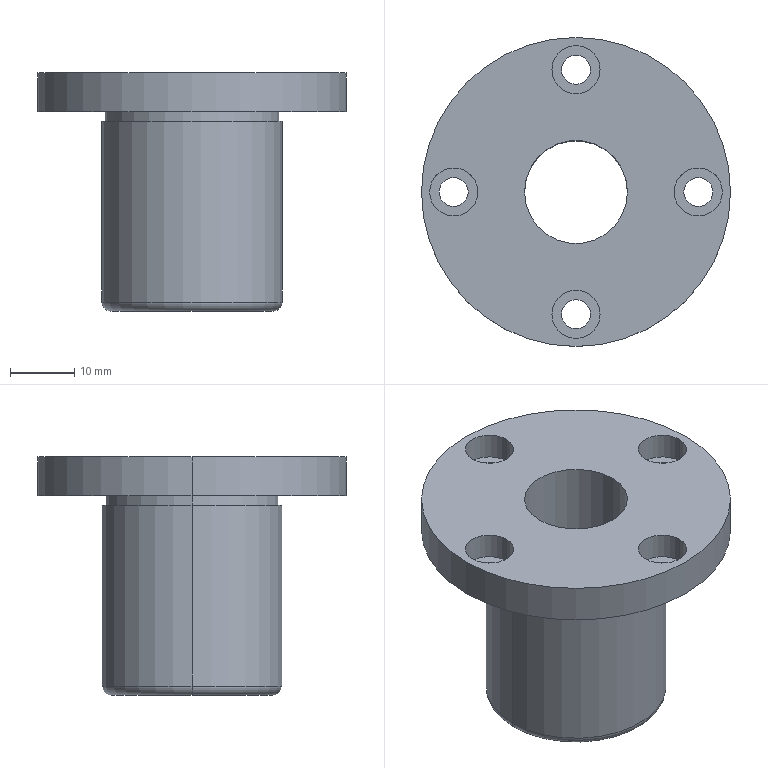Part | SolidWorks | features BaseBody 1 | 1 solid | 34 faces | box 48 x 48 x 37 mm | volume 21560 mm3 | cylinder 24 | plane 8 | torus 2 | commonest cylinder face diameters 4.5 x8 7.5 x8 16 x2 27 x2 28 x2 48 x2
STEP:
#1=CARTESIAN_POINT('',(-611.131,726.211,541.732));
#2=VERTEX_POINT('',#1);
#3=CARTESIAN_POINT('',(-595.131,726.211,541.732));
#4=VERTEX_POINT('',#3);
#5=CARTESIAN_POINT('',(-603.131,726.211,541.732));
#6=DIRECTION('',(0.,0.,1.));
#7=DIRECTION('',(-1.,0.,0.));
#8=AXIS2_PLACEMENT_3D('',#5,#6,#7);
#9=CIRCLE('',#8,8.);
#10=EDGE_CURVE('',#2,#4,#9,.T.);
#11=ORIENTED_EDGE('',*,*,#10,.T.);
#12=CARTESIAN_POINT('',(-595.131,726.211,504.732));
#13=VERTEX_POINT('',#12);
#14=CARTESIAN_POINT('',(-595.131,726.211,504.732));
#15=DIRECTION('',(0.,0.,1.));
#16=VECTOR('',#15,1000.);
#17=LINE('',#14,#16);
#18=EDGE_CURVE('',#13,#4,#17,.T.);
#19=ORIENTED_EDGE('',*,*,#18,.F.);
#20=CARTESIAN_POINT('',(-611.131,726.211,504.732));
#21=VERTEX_POINT('',#20);
#22=CARTESIAN_POINT('',(-603.131,726.211,504.732));
#23=DIRECTION('',(0.,0.,-1.));
#24=DIRECTION('',(1.,0.,0.));
#25=AXIS2_PLACEMENT_3D('',#22,#23,#24);
#26=CIRCLE('',#25,8.);
#27=EDGE_CURVE('',#13,#21,#26,.T.);
#28=ORIENTED_EDGE('',*,*,#27,.T.);
#29=CARTESIAN_POINT('',(-611.131,726.211,541.732));
#30=DIRECTION('',(0.,0.,-1.));
#31=VECTOR('',#30,1000.);
#32=LINE('',#29,#31);
#33=EDGE_CURVE('',#2,#21,#32,.T.);
#34=ORIENTED_EDGE('',*,*,#33,.F.);
#35=EDGE_LOOP('',(#11,#19,#28,#34));
#36=FACE_OUTER_BOUND('',#35,.T.);
#37=CARTESIAN_POINT('',(-603.131,726.211,504.732));
#38=DIRECTION('',(0.,0.,1.));
#39=DIRECTION('',(-1.,0.,0.));
#40=AXIS2_PLACEMENT_3D('',#37,#38,#39);
#41=CYLINDRICAL_SURFACE('',#40,8.);
#42=ADVANCED_FACE('',(#36),#41,.F.);
#43=ORIENTED_EDGE('',*,*,#18,.T.);
#44=CARTESIAN_POINT('',(-603.131,726.211,541.732));
#45=DIRECTION('',(0.,0.,1.));
#46=DIRECTION('',(1.,0.,0.));
#47=AXIS2_PLACEMENT_3D('',#44,#45,#46);
#48=CIRCLE('',#47,8.);
#49=EDGE_CURVE('',#4,#2,#48,.T.);
#50=ORIENTED_EDGE('',*,*,#49,.T.);
#51=ORIENTED_EDGE('',*,*,#33,.T.);
#52=CARTESIAN_POINT('',(-603.131,726.211,504.732));
#53=DIRECTION('',(0.,0.,-1.));
#54=DIRECTION('',(-1.,0.,0.));
#55=AXIS2_PLACEMENT_3D('',#52,#53,#54);
#56=CIRCLE('',#55,8.);
#57=EDGE_CURVE('',#21,#13,#56,.T.);
#58=ORIENTED_EDGE('',*,*,#57,.T.);
#59=EDGE_LOOP('',(#43,#50,#51,#58));
#60=FACE_OUTER_BOUND('',#59,.T.);
#61=CARTESIAN_POINT('',(-603.131,726.211,504.732));
#62=DIRECTION('',(0.,0.,1.));
#63=DIRECTION('',(-1.,0.,0.));
#64=AXIS2_PLACEMENT_3D('',#61,#62,#63);
#65=CYLINDRICAL_SURFACE('',#64,8.);
#66=ADVANCED_FACE('',(#60),#65,.F.);
#67=CARTESIAN_POINT('',(-590.531,726.211,504.732));
#68=VERTEX_POINT('',#67);
#69=CARTESIAN_POINT('',(-615.731,726.211,504.732));
#70=VERTEX_POINT('',#69);
#71=CARTESIAN_POINT('',(-603.131,726.211,504.732));
#72=DIRECTION('',(0.,0.,1.));
#73=DIRECTION('',(1.,0.,0.));
#74=AXIS2_PLACEMENT_3D('',#71,#72,#73);
#75=CIRCLE('',#74,12.6);
#76=EDGE_CURVE('',#68,#70,#75,.T.);
#77=ORIENTED_EDGE('',*,*,#76,.F.);
#78=CARTESIAN_POINT('',(-603.131,726.211,504.732));
#79=DIRECTION('',(0.,0.,1.));
#80=DIRECTION('',(-1.,0.,0.));
#81=AXIS2_PLACEMENT_3D('',#78,#79,#80);
#82=CIRCLE('',#81,12.6);
#83=EDGE_CURVE('',#70,#68,#82,.T.);
#84=ORIENTED_EDGE('',*,*,#83,.F.);
#85=EDGE_LOOP('',(#77,#84));
#86=FACE_OUTER_BOUND('',#85,.T.);
#87=ORIENTED_EDGE('',*,*,#57,.F.);
#88=ORIENTED_EDGE('',*,*,#27,.F.);
#89=EDGE_LOOP('',(#87,#88));
#90=FACE_BOUND('',#89,.T.);
#91=CARTESIAN_POINT('',(-603.131,734.211,504.732));
#92=DIRECTION('',(0.,0.,1.));
#93=DIRECTION('',(-1.,0.,0.));
#94=AXIS2_PLACEMENT_3D('',#91,#92,#93);
#95=PLANE('',#94);
#96=ADVANCED_FACE('',(#86,#90),#95,.F.);
#97=CARTESIAN_POINT('',(-589.131,726.211,506.132));
#98=VERTEX_POINT('',#97);
#99=CARTESIAN_POINT('',(-590.531,726.211,506.132));
#100=DIRECTION('',(0.,-1.,0.));
#101=DIRECTION('',(0.,0.,-1.));
#102=AXIS2_PLACEMENT_3D('',#99,#100,#101);
#103=CIRCLE('',#102,1.4);
#104=EDGE_CURVE('',#68,#98,#103,.T.);
#105=ORIENTED_EDGE('',*,*,#104,.T.);
#106=CARTESIAN_POINT('',(-617.131,726.211,506.132));
#107=VERTEX_POINT('',#106);
#108=CARTESIAN_POINT('',(-603.131,726.211,506.132));
#109=DIRECTION('',(0.,0.,1.));
#110=DIRECTION('',(-1.,0.,0.));
#111=AXIS2_PLACEMENT_3D('',#108,#109,#110);
#112=CIRCLE('',#111,14.);
#113=EDGE_CURVE('',#107,#98,#112,.T.);
#114=ORIENTED_EDGE('',*,*,#113,.F.);
#115=CARTESIAN_POINT('',(-615.731,726.211,506.132));
#116=DIRECTION('',(0.,-1.,0.));
#117=DIRECTION('',(-1.,0.,0.));
#118=AXIS2_PLACEMENT_3D('',#115,#116,#117);
#119=CIRCLE('',#118,1.4);
#120=EDGE_CURVE('',#107,#70,#119,.T.);
#121=ORIENTED_EDGE('',*,*,#120,.T.);
#122=ORIENTED_EDGE('',*,*,#83,.T.);
#123=EDGE_LOOP('',(#105,#114,#121,#122));
#124=FACE_OUTER_BOUND('',#123,.T.);
#125=CARTESIAN_POINT('',(-603.131,726.211,506.132));
#126=DIRECTION('',(0.,0.,1.));
#127=DIRECTION('',(-1.,0.,0.));
#128=AXIS2_PLACEMENT_3D('',#125,#126,#127);
#129=TOROIDAL_SURFACE('',#128,12.6,1.4);
#130=ADVANCED_FACE('',(#124),#129,.T.);
#131=CARTESIAN_POINT('',(-603.131,726.211,506.132));
#132=DIRECTION('',(0.,0.,1.));
#133=DIRECTION('',(1.,0.,0.));
#134=AXIS2_PLACEMENT_3D('',#131,#132,#133);
#135=CIRCLE('',#134,14.);
#136=EDGE_CURVE('',#98,#107,#135,.T.);
#137=ORIENTED_EDGE('',*,*,#136,.F.);
#138=ORIENTED_EDGE('',*,*,#104,.F.);
#139=ORIENTED_EDGE('',*,*,#76,.T.);
#140=ORIENTED_EDGE('',*,*,#120,.F.);
#141=EDGE_LOOP('',(#137,#138,#139,#140));
#142=FACE_OUTER_BOUND('',#141,.T.);
#143=CARTESIAN_POINT('',(-603.131,726.211,506.132));
#144=DIRECTION('',(0.,0.,1.));
#145=DIRECTION('',(-1.,0.,0.));
#146=AXIS2_PLACEMENT_3D('',#143,#144,#145);
#147=TOROIDAL_SURFACE('',#146,12.6,1.4);
#148=ADVANCED_FACE('',(#142),#147,.T.);
#149=CARTESIAN_POINT('',(-617.131,726.211,534.232));
#150=VERTEX_POINT('',#149);
#151=CARTESIAN_POINT('',(-589.131,726.211,534.232));
#152=VERTEX_POINT('',#151);
#153=CARTESIAN_POINT('',(-603.131,726.211,534.232));
#154=DIRECTION('',(0.,0.,-1.));
#155=DIRECTION('',(-1.,0.,0.));
#156=AXIS2_PLACEMENT_3D('',#153,#154,#155);
#157=CIRCLE('',#156,14.);
#158=EDGE_CURVE('',#150,#152,#157,.T.);
#159=ORIENTED_EDGE('',*,*,#158,.T.);
#160=CARTESIAN_POINT('',(-589.131,726.211,534.232));
#161=DIRECTION('',(0.,0.,-1.));
#162=VECTOR('',#161,1000.);
#163=LINE('',#160,#162);
#164=EDGE_CURVE('',#152,#98,#163,.T.);
#165=ORIENTED_EDGE('',*,*,#164,.T.);
#166=ORIENTED_EDGE('',*,*,#136,.T.);
#167=CARTESIAN_POINT('',(-617.131,726.211,506.132));
#168=DIRECTION('',(0.,0.,1.));
#169=VECTOR('',#168,1000.);
#170=LINE('',#167,#169);
#171=EDGE_CURVE('',#107,#150,#170,.T.);
#172=ORIENTED_EDGE('',*,*,#171,.T.);
#173=EDGE_LOOP('',(#159,#165,#166,#172));
#174=FACE_OUTER_BOUND('',#173,.T.);
#175=CARTESIAN_POINT('',(-603.131,726.211,504.732));
#176=DIRECTION('',(0.,0.,1.));
#177=DIRECTION('',(-1.,0.,0.));
#178=AXIS2_PLACEMENT_3D('',#175,#176,#177);
#179=CYLINDRICAL_SURFACE('',#178,14.);
#180=ADVANCED_FACE('',(#174),#179,.T.);
#181=ORIENTED_EDGE('',*,*,#164,.F.);
#182=CARTESIAN_POINT('',(-603.131,726.211,534.232));
#183=DIRECTION('',(0.,0.,-1.));
#184=DIRECTION('',(1.,0.,0.));
#185=AXIS2_PLACEMENT_3D('',#182,#183,#184);
#186=CIRCLE('',#185,14.);
#187=EDGE_CURVE('',#152,#150,#186,.T.);
#188=ORIENTED_EDGE('',*,*,#187,.T.);
#189=ORIENTED_EDGE('',*,*,#171,.F.);
#190=ORIENTED_EDGE('',*,*,#113,.T.);
#191=EDGE_LOOP('',(#181,#188,#189,#190));
#192=FACE_OUTER_BOUND('',#191,.T.);
#193=CARTESIAN_POINT('',(-603.131,726.211,504.732));
#194=DIRECTION('',(0.,0.,1.));
#195=DIRECTION('',(-1.,0.,0.));
#196=AXIS2_PLACEMENT_3D('',#193,#194,#195);
#197=CYLINDRICAL_SURFACE('',#196,14.);
#198=ADVANCED_FACE('',(#192),#197,.T.);
#199=ORIENTED_EDGE('',*,*,#158,.F.);
#200=ORIENTED_EDGE('',*,*,#187,.F.);
#201=EDGE_LOOP('',(#199,#200));
#202=FACE_OUTER_BOUND('',#201,.T.);
#203=CARTESIAN_POINT('',(-589.631,726.211,534.232));
#204=VERTEX_POINT('',#203);
#205=CARTESIAN_POINT('',(-616.631,726.211,534.232));
#206=VERTEX_POINT('',#205);
#207=CARTESIAN_POINT('',(-603.131,726.211,534.232));
#208=DIRECTION('',(0.,0.,1.));
#209=DIRECTION('',(1.,0.,0.));
#210=AXIS2_PLACEMENT_3D('',#207,#208,#209);
#211=CIRCLE('',#210,13.5);
#212=EDGE_CURVE('',#204,#206,#211,.T.);
#213=ORIENTED_EDGE('',*,*,#212,.F.);
#214=CARTESIAN_POINT('',(-603.131,726.211,534.232));
#215=DIRECTION('',(0.,0.,1.));
#216=DIRECTION('',(-1.,0.,0.));
#217=AXIS2_PLACEMENT_3D('',#214,#215,#216);
#218=CIRCLE('',#217,13.5);
#219=EDGE_CURVE('',#206,#204,#218,.T.);
#220=ORIENTED_EDGE('',*,*,#219,.F.);
#221=EDGE_LOOP('',(#213,#220));
#222=FACE_BOUND('',#221,.T.);
#223=CARTESIAN_POINT('',(-603.131,740.211,534.232));
#224=DIRECTION('',(0.,0.,-1.));
#225=DIRECTION('',(1.,0.,0.));
#226=AXIS2_PLACEMENT_3D('',#223,#224,#225);
#227=PLANE('',#226);
#228=ADVANCED_FACE('',(#202,#222),#227,.F.);
#229=CARTESIAN_POINT('',(-589.631,726.211,535.732));
#230=VERTEX_POINT('',#229);
#231=CARTESIAN_POINT('',(-589.631,726.211,534.232));
#232=DIRECTION('',(0.,0.,1.));
#233=VECTOR('',#232,1000.);
#234=LINE('',#231,#233);
#235=EDGE_CURVE('',#204,#230,#234,.T.);
#236=ORIENTED_EDGE('',*,*,#235,.T.);
#237=CARTESIAN_POINT('',(-616.631,726.211,535.732));
#238=VERTEX_POINT('',#237);
#239=CARTESIAN_POINT('',(-603.131,726.211,535.732));
#240=DIRECTION('',(0.,0.,-1.));
#241=DIRECTION('',(1.,0.,0.));
#242=AXIS2_PLACEMENT_3D('',#239,#240,#241);
#243=CIRCLE('',#242,13.5);
#244=EDGE_CURVE('',#230,#238,#243,.T.);
#245=ORIENTED_EDGE('',*,*,#244,.T.);
#246=CARTESIAN_POINT('',(-616.631,726.211,535.732));
#247=DIRECTION('',(0.,0.,-1.));
#248=VECTOR('',#247,1000.);
#249=LINE('',#246,#248);
#250=EDGE_CURVE('',#238,#206,#249,.T.);
#251=ORIENTED_EDGE('',*,*,#250,.T.);
#252=ORIENTED_EDGE('',*,*,#219,.T.);
#253=EDGE_LOOP('',(#236,#245,#251,#252));
#254=FACE_OUTER_BOUND('',#253,.T.);
#255=CARTESIAN_POINT('',(-603.131,726.211,504.732));
#256=DIRECTION('',(0.,0.,1.));
#257=DIRECTION('',(-1.,0.,0.));
#258=AXIS2_PLACEMENT_3D('',#255,#256,#257);
#259=CYLINDRICAL_SURFACE('',#258,13.5);
#260=ADVANCED_FACE('',(#254),#259,.T.);
#261=CARTESIAN_POINT('',(-603.131,726.211,535.732));
#262=DIRECTION('',(0.,0.,-1.));
#263=DIRECTION('',(-1.,0.,0.));
#264=AXIS2_PLACEMENT_3D('',#261,#262,#263);
#265=CIRCLE('',#264,13.5);
#266=EDGE_CURVE('',#238,#230,#265,.T.);
#267=ORIENTED_EDGE('',*,*,#266,.T.);
#268=ORIENTED_EDGE('',*,*,#235,.F.);
#269=ORIENTED_EDGE('',*,*,#212,.T.);
#270=ORIENTED_EDGE('',*,*,#250,.F.);
#271=EDGE_LOOP('',(#267,#268,#269,#270));
#272=FACE_OUTER_BOUND('',#271,.T.);
#273=CARTESIAN_POINT('',(-603.131,726.211,504.732));
#274=DIRECTION('',(0.,0.,1.));
#275=DIRECTION('',(-1.,0.,0.));
#276=AXIS2_PLACEMENT_3D('',#273,#274,#275);
#277=CYLINDRICAL_SURFACE('',#276,13.5);
#278=ADVANCED_FACE('',(#272),#277,.T.);
#279=CARTESIAN_POINT('',(-579.131,726.211,535.732));
#280=VERTEX_POINT('',#279);
#281=CARTESIAN_POINT('',(-627.131,726.211,535.732));
#282=VERTEX_POINT('',#281);
#283=CARTESIAN_POINT('',(-603.131,726.211,535.732));
#284=DIRECTION('',(0.,0.,1.));
#285=DIRECTION('',(1.,0.,0.));
#286=AXIS2_PLACEMENT_3D('',#283,#284,#285);
#287=CIRCLE('',#286,24.);
#288=EDGE_CURVE('',#280,#282,#287,.T.);
#289=ORIENTED_EDGE('',*,*,#288,.F.);
#290=CARTESIAN_POINT('',(-603.131,726.211,535.732));
#291=DIRECTION('',(0.,0.,1.));
#292=DIRECTION('',(-1.,0.,0.));
#293=AXIS2_PLACEMENT_3D('',#290,#291,#292);
#294=CIRCLE('',#293,24.);
#295=EDGE_CURVE('',#282,#280,#294,.T.);
#296=ORIENTED_EDGE('',*,*,#295,.F.);
#297=EDGE_LOOP('',(#289,#296));
#298=FACE_OUTER_BOUND('',#297,.T.);
#299=CARTESIAN_POINT('',(-624.381,726.211,535.732));
#300=VERTEX_POINT('',#299);
#301=CARTESIAN_POINT('',(-619.881,726.211,535.732));
#302=VERTEX_POINT('',#301);
#303=CARTESIAN_POINT('',(-622.131,726.211,535.732));
#304=DIRECTION('',(0.,0.,-1.));
#305=DIRECTION('',(-1.,0.,0.));
#306=AXIS2_PLACEMENT_3D('',#303,#304,#305);
#307=CIRCLE('',#306,2.25);
#308=EDGE_CURVE('',#300,#302,#307,.T.);
#309=ORIENTED_EDGE('',*,*,#308,.F.);
#310=CARTESIAN_POINT('',(-622.131,726.211,535.732));
#311=DIRECTION('',(0.,0.,-1.));
#312=DIRECTION('',(1.,0.,0.));
#313=AXIS2_PLACEMENT_3D('',#310,#311,#312);
#314=CIRCLE('',#313,2.25);
#315=EDGE_CURVE('',#302,#300,#314,.T.);
#316=ORIENTED_EDGE('',*,*,#315,.F.);
#317=EDGE_LOOP('',(#309,#316));
#318=FACE_BOUND('',#317,.T.);
#319=CARTESIAN_POINT('',(-605.381,745.211,535.732));
#320=VERTEX_POINT('',#319);
#321=CARTESIAN_POINT('',(-600.881,745.211,535.732));
#322=VERTEX_POINT('',#321);
#323=CARTESIAN_POINT('',(-603.131,745.211,535.732));
#324=DIRECTION('',(0.,0.,-1.));
#325=DIRECTION('',(-1.,0.,0.));
#326=AXIS2_PLACEMENT_3D('',#323,#324,#325);
#327=CIRCLE('',#326,2.25);
#328=EDGE_CURVE('',#320,#322,#327,.T.);
#329=ORIENTED_EDGE('',*,*,#328,.F.);
#330=CARTESIAN_POINT('',(-603.131,745.211,535.732));
#331=DIRECTION('',(0.,0.,-1.));
#332=DIRECTION('',(1.,0.,0.));
#333=AXIS2_PLACEMENT_3D('',#330,#331,#332);
#334=CIRCLE('',#333,2.25);
#335=EDGE_CURVE('',#322,#320,#334,.T.);
#336=ORIENTED_EDGE('',*,*,#335,.F.);
#337=EDGE_LOOP('',(#329,#336));
#338=FACE_BOUND('',#337,.T.);
#339=ORIENTED_EDGE('',*,*,#266,.F.);
#340=ORIENTED_EDGE('',*,*,#244,.F.);
#341=EDGE_LOOP('',(#339,#340));
#342=FACE_BOUND('',#341,.T.);
#343=CARTESIAN_POINT('',(-605.381,707.211,535.732));
#344=VERTEX_POINT('',#343);
#345=CARTESIAN_POINT('',(-600.881,707.211,535.732));
#346=VERTEX_POINT('',#345);
#347=CARTESIAN_POINT('',(-603.131,707.211,535.732));
#348=DIRECTION('',(0.,0.,-1.));
#349=DIRECTION('',(-1.,0.,0.));
#350=AXIS2_PLACEMENT_3D('',#347,#348,#349);
#351=CIRCLE('',#350,2.25);
#352=EDGE_CURVE('',#344,#346,#351,.T.);
#353=ORIENTED_EDGE('',*,*,#352,.F.);
#354=CARTESIAN_POINT('',(-603.131,707.211,535.732));
#355=DIRECTION('',(0.,0.,-1.));
#356=DIRECTION('',(1.,0.,0.));
#357=AXIS2_PLACEMENT_3D('',#354,#355,#356);
#358=CIRCLE('',#357,2.25);
#359=EDGE_CURVE('',#346,#344,#358,.T.);
#360=ORIENTED_EDGE('',*,*,#359,.F.);
#361=EDGE_LOOP('',(#353,#360));
#362=FACE_BOUND('',#361,.T.);
#363=CARTESIAN_POINT('',(-586.381,726.211,535.732));
#364=VERTEX_POINT('',#363);
#365=CARTESIAN_POINT('',(-581.881,726.211,535.732));
#366=VERTEX_POINT('',#365);
#367=CARTESIAN_POINT('',(-584.131,726.211,535.732));
#368=DIRECTION('',(0.,0.,-1.));
#369=DIRECTION('',(-1.,0.,0.));
#370=AXIS2_PLACEMENT_3D('',#367,#368,#369);
#371=CIRCLE('',#370,2.25);
#372=EDGE_CURVE('',#364,#366,#371,.T.);
#373=ORIENTED_EDGE('',*,*,#372,.F.);
#374=CARTESIAN_POINT('',(-584.131,726.211,535.732));
#375=DIRECTION('',(0.,0.,-1.));
#376=DIRECTION('',(1.,0.,0.));
#377=AXIS2_PLACEMENT_3D('',#374,#375,#376);
#378=CIRCLE('',#377,2.25);
#379=EDGE_CURVE('',#366,#364,#378,.T.);
#380=ORIENTED_EDGE('',*,*,#379,.F.);
#381=EDGE_LOOP('',(#373,#380));
#382=FACE_BOUND('',#381,.T.);
#383=CARTESIAN_POINT('',(-603.131,739.711,535.732));
#384=DIRECTION('',(0.,0.,1.));
#385=DIRECTION('',(-1.,0.,0.));
#386=AXIS2_PLACEMENT_3D('',#383,#384,#385);
#387=PLANE('',#386);
#388=ADVANCED_FACE('',(#298,#318,#338,#342,#362,#382),#387,.F.);
#389=CARTESIAN_POINT('',(-579.131,726.211,541.732));
#390=VERTEX_POINT('',#389);
#391=CARTESIAN_POINT('',(-579.131,726.211,535.732));
#392=DIRECTION('',(0.,0.,1.));
#393=VECTOR('',#392,1000.);
#394=LINE('',#391,#393);
#395=EDGE_CURVE('',#280,#390,#394,.T.);
#396=ORIENTED_EDGE('',*,*,#395,.T.);
#397=CARTESIAN_POINT('',(-627.131,726.211,541.732));
#398=VERTEX_POINT('',#397);
#399=CARTESIAN_POINT('',(-603.131,726.211,541.732));
#400=DIRECTION('',(0.,0.,-1.));
#401=DIRECTION('',(1.,0.,0.));
#402=AXIS2_PLACEMENT_3D('',#399,#400,#401);
#403=CIRCLE('',#402,24.);
#404=EDGE_CURVE('',#390,#398,#403,.T.);
#405=ORIENTED_EDGE('',*,*,#404,.T.);
#406=CARTESIAN_POINT('',(-627.131,726.211,541.732));
#407=DIRECTION('',(0.,0.,-1.));
#408=VECTOR('',#407,1000.);
#409=LINE('',#406,#408);
#410=EDGE_CURVE('',#398,#282,#409,.T.);
#411=ORIENTED_EDGE('',*,*,#410,.T.);
#412=ORIENTED_EDGE('',*,*,#295,.T.);
#413=EDGE_LOOP('',(#396,#405,#411,#412));
#414=FACE_OUTER_BOUND('',#413,.T.);
#415=CARTESIAN_POINT('',(-603.131,726.211,504.732));
#416=DIRECTION('',(0.,0.,1.));
#417=DIRECTION('',(-1.,0.,0.));
#418=AXIS2_PLACEMENT_3D('',#415,#416,#417);
#419=CYLINDRICAL_SURFACE('',#418,24.);
#420=ADVANCED_FACE('',(#414),#419,.T.);
#421=CARTESIAN_POINT('',(-603.131,726.211,541.732));
#422=DIRECTION('',(0.,0.,-1.));
#423=DIRECTION('',(-1.,0.,0.));
#424=AXIS2_PLACEMENT_3D('',#421,#422,#423);
#425=CIRCLE('',#424,24.);
#426=EDGE_CURVE('',#398,#390,#425,.T.);
#427=ORIENTED_EDGE('',*,*,#426,.T.);
#428=ORIENTED_EDGE('',*,*,#395,.F.);
#429=ORIENTED_EDGE('',*,*,#288,.T.);
#430=ORIENTED_EDGE('',*,*,#410,.F.);
#431=EDGE_LOOP('',(#427,#428,#429,#430));
#432=FACE_OUTER_BOUND('',#431,.T.);
#433=CARTESIAN_POINT('',(-603.131,726.211,504.732));
#434=DIRECTION('',(0.,0.,1.));
#435=DIRECTION('',(-1.,0.,0.));
#436=AXIS2_PLACEMENT_3D('',#433,#434,#435);
#437=CYLINDRICAL_SURFACE('',#436,24.);
#438=ADVANCED_FACE('',(#432),#437,.T.);
#439=ORIENTED_EDGE('',*,*,#426,.F.);
#440=ORIENTED_EDGE('',*,*,#404,.F.);
#441=EDGE_LOOP('',(#439,#440));
#442=FACE_OUTER_BOUND('',#441,.T.);
#443=CARTESIAN_POINT('',(-618.381,726.211,541.732));
#444=VERTEX_POINT('',#443);
#445=CARTESIAN_POINT('',(-625.881,726.211,541.732));
#446=VERTEX_POINT('',#445);
#447=CARTESIAN_POINT('',(-622.131,726.211,541.732));
#448=DIRECTION('',(0.,0.,1.));
#449=DIRECTION('',(1.,0.,0.));
#450=AXIS2_PLACEMENT_3D('',#447,#448,#449);
#451=CIRCLE('',#450,3.75);
#452=EDGE_CURVE('',#444,#446,#451,.T.);
#453=ORIENTED_EDGE('',*,*,#452,.F.);
#454=CARTESIAN_POINT('',(-622.131,726.211,541.732));
#455=DIRECTION('',(0.,0.,1.));
#456=DIRECTION('',(-1.,0.,0.));
#457=AXIS2_PLACEMENT_3D('',#454,#455,#456);
#458=CIRCLE('',#457,3.75);
#459=EDGE_CURVE('',#446,#444,#458,.T.);
#460=ORIENTED_EDGE('',*,*,#459,.F.);
#461=EDGE_LOOP('',(#453,#460));
#462=FACE_BOUND('',#461,.T.);
#463=CARTESIAN_POINT('',(-599.381,745.211,541.732));
#464=VERTEX_POINT('',#463);
#465=CARTESIAN_POINT('',(-606.881,745.211,541.732));
#466=VERTEX_POINT('',#465);
#467=CARTESIAN_POINT('',(-603.131,745.211,541.732));
#468=DIRECTION('',(0.,0.,1.));
#469=DIRECTION('',(1.,0.,0.));
#470=AXIS2_PLACEMENT_3D('',#467,#468,#469);
#471=CIRCLE('',#470,3.75);
#472=EDGE_CURVE('',#464,#466,#471,.T.);
#473=ORIENTED_EDGE('',*,*,#472,.F.);
#474=CARTESIAN_POINT('',(-603.131,745.211,541.732));
#475=DIRECTION('',(0.,0.,1.));
#476=DIRECTION('',(-1.,0.,0.));
#477=AXIS2_PLACEMENT_3D('',#474,#475,#476);
#478=CIRCLE('',#477,3.75);
#479=EDGE_CURVE('',#466,#464,#478,.T.);
#480=ORIENTED_EDGE('',*,*,#479,.F.);
#481=EDGE_LOOP('',(#473,#480));
#482=FACE_BOUND('',#481,.T.);
#483=ORIENTED_EDGE('',*,*,#49,.F.);
#484=ORIENTED_EDGE('',*,*,#10,.F.);
#485=EDGE_LOOP('',(#483,#484));
#486=FACE_BOUND('',#485,.T.);
#487=CARTESIAN_POINT('',(-599.381,707.211,541.732));
#488=VERTEX_POINT('',#487);
#489=CARTESIAN_POINT('',(-606.881,707.211,541.732));
#490=VERTEX_POINT('',#489);
#491=CARTESIAN_POINT('',(-603.131,707.211,541.732));
#492=DIRECTION('',(0.,0.,1.));
#493=DIRECTION('',(1.,0.,0.));
#494=AXIS2_PLACEMENT_3D('',#491,#492,#493);
#495=CIRCLE('',#494,3.75);
#496=EDGE_CURVE('',#488,#490,#495,.T.);
#497=ORIENTED_EDGE('',*,*,#496,.F.);
#498=CARTESIAN_POINT('',(-603.131,707.211,541.732));
#499=DIRECTION('',(0.,0.,1.));
#500=DIRECTION('',(-1.,0.,0.));
#501=AXIS2_PLACEMENT_3D('',#498,#499,#500);
#502=CIRCLE('',#501,3.75);
#503=EDGE_CURVE('',#490,#488,#502,.T.);
#504=ORIENTED_EDGE('',*,*,#503,.F.);
#505=EDGE_LOOP('',(#497,#504));
#506=FACE_BOUND('',#505,.T.);
#507=CARTESIAN_POINT('',(-580.381,726.211,541.732));
#508=VERTEX_POINT('',#507);
#509=CARTESIAN_POINT('',(-587.881,726.211,541.732));
#510=VERTEX_POINT('',#509);
#511=CARTESIAN_POINT('',(-584.131,726.211,541.732));
#512=DIRECTION('',(0.,0.,1.));
#513=DIRECTION('',(1.,0.,0.));
#514=AXIS2_PLACEMENT_3D('',#511,#512,#513);
#515=CIRCLE('',#514,3.75);
#516=EDGE_CURVE('',#508,#510,#515,.T.);
#517=ORIENTED_EDGE('',*,*,#516,.F.);
#518=CARTESIAN_POINT('',(-584.131,726.211,541.732));
#519=DIRECTION('',(0.,0.,1.));
#520=DIRECTION('',(-1.,0.,0.));
#521=AXIS2_PLACEMENT_3D('',#518,#519,#520);
#522=CIRCLE('',#521,3.75);
#523=EDGE_CURVE('',#510,#508,#522,.T.);
#524=ORIENTED_EDGE('',*,*,#523,.F.);
#525=EDGE_LOOP('',(#517,#524));
#526=FACE_BOUND('',#525,.T.);
#527=CARTESIAN_POINT('',(-603.131,750.211,541.732));
#528=DIRECTION('',(0.,0.,-1.));
#529=DIRECTION('',(1.,0.,0.));
#530=AXIS2_PLACEMENT_3D('',#527,#528,#529);
#531=PLANE('',#530);
#532=ADVANCED_FACE('',(#442,#462,#482,#486,#506,#526),#531,.F.);
#533=ORIENTED_EDGE('',*,*,#459,.T.);
#534=CARTESIAN_POINT('',(-618.381,726.211,537.632));
#535=VERTEX_POINT('',#534);
#536=CARTESIAN_POINT('',(-618.381,726.211,541.732));
#537=DIRECTION('',(0.,0.,-1.));
#538=VECTOR('',#537,1000.);
#539=LINE('',#536,#538);
#540=EDGE_CURVE('',#444,#535,#539,.T.);
#541=ORIENTED_EDGE('',*,*,#540,.T.);
#542=CARTESIAN_POINT('',(-625.881,726.211,537.632));
#543=VERTEX_POINT('',#542);
#544=CARTESIAN_POINT('',(-622.131,726.211,537.632));
#545=DIRECTION('',(0.,0.,-1.));
#546=DIRECTION('',(1.,0.,0.));
#547=AXIS2_PLACEMENT_3D('',#544,#545,#546);
#548=CIRCLE('',#547,3.75);
#549=EDGE_CURVE('',#535,#543,#548,.T.);
#550=ORIENTED_EDGE('',*,*,#549,.T.);
#551=CARTESIAN_POINT('',(-625.881,726.211,537.632));
#552=DIRECTION('',(0.,0.,1.));
#553=VECTOR('',#552,1000.);
#554=LINE('',#551,#553);
#555=EDGE_CURVE('',#543,#446,#554,.T.);
#556=ORIENTED_EDGE('',*,*,#555,.T.);
#557=EDGE_LOOP('',(#533,#541,#550,#556));
#558=FACE_OUTER_BOUND('',#557,.T.);
#559=CARTESIAN_POINT('',(-622.131,726.211,535.732));
#560=DIRECTION('',(0.,0.,1.));
#561=DIRECTION('',(-1.,0.,0.));
#562=AXIS2_PLACEMENT_3D('',#559,#560,#561);
#563=CYLINDRICAL_SURFACE('',#562,3.75);
#564=ADVANCED_FACE('',(#558),#563,.F.);
#565=ORIENTED_EDGE('',*,*,#540,.F.);
#566=ORIENTED_EDGE('',*,*,#452,.T.);
#567=ORIENTED_EDGE('',*,*,#555,.F.);
#568=CARTESIAN_POINT('',(-622.131,726.211,537.632));
#569=DIRECTION('',(0.,0.,-1.));
#570=DIRECTION('',(-1.,0.,0.));
#571=AXIS2_PLACEMENT_3D('',#568,#569,#570);
#572=CIRCLE('',#571,3.75);
#573=EDGE_CURVE('',#543,#535,#572,.T.);
#574=ORIENTED_EDGE('',*,*,#573,.T.);
#575=EDGE_LOOP('',(#565,#566,#567,#574));
#576=FACE_OUTER_BOUND('',#575,.T.);
#577=CARTESIAN_POINT('',(-622.131,726.211,535.732));
#578=DIRECTION('',(0.,0.,1.));
#579=DIRECTION('',(-1.,0.,0.));
#580=AXIS2_PLACEMENT_3D('',#577,#578,#579);
#581=CYLINDRICAL_SURFACE('',#580,3.75);
#582=ADVANCED_FACE('',(#576),#581,.F.);
#583=ORIENTED_EDGE('',*,*,#573,.F.);
#584=ORIENTED_EDGE('',*,*,#549,.F.);
#585=EDGE_LOOP('',(#583,#584));
#586=FACE_OUTER_BOUND('',#585,.T.);
#587=CARTESIAN_POINT('',(-619.881,726.211,537.632));
#588=VERTEX_POINT('',#587);
#589=CARTESIAN_POINT('',(-624.381,726.211,537.632));
#590=VERTEX_POINT('',#589);
#591=CARTESIAN_POINT('',(-622.131,726.211,537.632));
#592=DIRECTION('',(0.,0.,1.));
#593=DIRECTION('',(1.,0.,0.));
#594=AXIS2_PLACEMENT_3D('',#591,#592,#593);
#595=CIRCLE('',#594,2.25);
#596=EDGE_CURVE('',#588,#590,#595,.T.);
#597=ORIENTED_EDGE('',*,*,#596,.F.);
#598=CARTESIAN_POINT('',(-622.131,726.211,537.632));
#599=DIRECTION('',(0.,0.,1.));
#600=DIRECTION('',(-1.,0.,0.));
#601=AXIS2_PLACEMENT_3D('',#598,#599,#600);
#602=CIRCLE('',#601,2.25);
#603=EDGE_CURVE('',#590,#588,#602,.T.);
#604=ORIENTED_EDGE('',*,*,#603,.F.);
#605=EDGE_LOOP('',(#597,#604));
#606=FACE_BOUND('',#605,.T.);
#607=CARTESIAN_POINT('',(-625.881,726.211,537.632));
#608=DIRECTION('',(0.,0.,1.));
#609=DIRECTION('',(-1.,0.,0.));
#610=AXIS2_PLACEMENT_3D('',#607,#608,#609);
#611=PLANE('',#610);
#612=ADVANCED_FACE('',(#586,#606),#611,.T.);
#613=ORIENTED_EDGE('',*,*,#603,.T.);
#614=CARTESIAN_POINT('',(-619.881,726.211,537.632));
#615=DIRECTION('',(0.,0.,-1.));
#616=VECTOR('',#615,1000.);
#617=LINE('',#614,#616);
#618=EDGE_CURVE('',#588,#302,#617,.T.);
#619=ORIENTED_EDGE('',*,*,#618,.T.);
#620=ORIENTED_EDGE('',*,*,#315,.T.);
#621=CARTESIAN_POINT('',(-624.381,726.211,535.732));
#622=DIRECTION('',(0.,0.,1.));
#623=VECTOR('',#622,1000.);
#624=LINE('',#621,#623);
#625=EDGE_CURVE('',#300,#590,#624,.T.);
#626=ORIENTED_EDGE('',*,*,#625,.T.);
#627=EDGE_LOOP('',(#613,#619,#620,#626));
#628=FACE_OUTER_BOUND('',#627,.T.);
#629=CARTESIAN_POINT('',(-622.131,726.211,535.732));
#630=DIRECTION('',(0.,0.,1.));
#631=DIRECTION('',(-1.,0.,0.));
#632=AXIS2_PLACEMENT_3D('',#629,#630,#631);
#633=CYLINDRICAL_SURFACE('',#632,2.25);
#634=ADVANCED_FACE('',(#628),#633,.F.);
#635=ORIENTED_EDGE('',*,*,#618,.F.);
#636=ORIENTED_EDGE('',*,*,#596,.T.);
#637=ORIENTED_EDGE('',*,*,#625,.F.);
#638=ORIENTED_EDGE('',*,*,#308,.T.);
#639=EDGE_LOOP('',(#635,#636,#637,#638));
#640=FACE_OUTER_BOUND('',#639,.T.);
#641=CARTESIAN_POINT('',(-622.131,726.211,535.732));
#642=DIRECTION('',(0.,0.,1.));
#643=DIRECTION('',(-1.,0.,0.));
#644=AXIS2_PLACEMENT_3D('',#641,#642,#643);
#645=CYLINDRICAL_SURFACE('',#644,2.25);
#646=ADVANCED_FACE('',(#640),#645,.F.);
#647=ORIENTED_EDGE('',*,*,#479,.T.);
#648=CARTESIAN_POINT('',(-599.381,745.211,537.632));
#649=VERTEX_POINT('',#648);
#650=CARTESIAN_POINT('',(-599.381,745.211,541.732));
#651=DIRECTION('',(0.,0.,-1.));
#652=VECTOR('',#651,1000.);
#653=LINE('',#650,#652);
#654=EDGE_CURVE('',#464,#649,#653,.T.);
#655=ORIENTED_EDGE('',*,*,#654,.T.);
#656=CARTESIAN_POINT('',(-606.881,745.211,537.632));
#657=VERTEX_POINT('',#656);
#658=CARTESIAN_POINT('',(-603.131,745.211,537.632));
#659=DIRECTION('',(0.,0.,-1.));
#660=DIRECTION('',(1.,0.,0.));
#661=AXIS2_PLACEMENT_3D('',#658,#659,#660);
#662=CIRCLE('',#661,3.75);
#663=EDGE_CURVE('',#649,#657,#662,.T.);
#664=ORIENTED_EDGE('',*,*,#663,.T.);
#665=CARTESIAN_POINT('',(-606.881,745.211,537.632));
#666=DIRECTION('',(0.,0.,1.));
#667=VECTOR('',#666,1000.);
#668=LINE('',#665,#667);
#669=EDGE_CURVE('',#657,#466,#668,.T.);
#670=ORIENTED_EDGE('',*,*,#669,.T.);
#671=EDGE_LOOP('',(#647,#655,#664,#670));
#672=FACE_OUTER_BOUND('',#671,.T.);
#673=CARTESIAN_POINT('',(-603.131,745.211,535.732));
#674=DIRECTION('',(0.,0.,1.));
#675=DIRECTION('',(-1.,0.,0.));
#676=AXIS2_PLACEMENT_3D('',#673,#674,#675);
#677=CYLINDRICAL_SURFACE('',#676,3.75);
#678=ADVANCED_FACE('',(#672),#677,.F.);
#679=ORIENTED_EDGE('',*,*,#654,.F.);
#680=ORIENTED_EDGE('',*,*,#472,.T.);
#681=ORIENTED_EDGE('',*,*,#669,.F.);
#682=CARTESIAN_POINT('',(-603.131,745.211,537.632));
#683=DIRECTION('',(0.,0.,-1.));
#684=DIRECTION('',(-1.,0.,0.));
#685=AXIS2_PLACEMENT_3D('',#682,#683,#684);
#686=CIRCLE('',#685,3.75);
#687=EDGE_CURVE('',#657,#649,#686,.T.);
#688=ORIENTED_EDGE('',*,*,#687,.T.);
#689=EDGE_LOOP('',(#679,#680,#681,#688));
#690=FACE_OUTER_BOUND('',#689,.T.);
#691=CARTESIAN_POINT('',(-603.131,745.211,535.732));
#692=DIRECTION('',(0.,0.,1.));
#693=DIRECTION('',(-1.,0.,0.));
#694=AXIS2_PLACEMENT_3D('',#691,#692,#693);
#695=CYLINDRICAL_SURFACE('',#694,3.75);
#696=ADVANCED_FACE('',(#690),#695,.F.);
#697=ORIENTED_EDGE('',*,*,#687,.F.);
#698=ORIENTED_EDGE('',*,*,#663,.F.);
#699=EDGE_LOOP('',(#697,#698));
#700=FACE_OUTER_BOUND('',#699,.T.);
#701=CARTESIAN_POINT('',(-600.881,745.211,537.632));
#702=VERTEX_POINT('',#701);
#703=CARTESIAN_POINT('',(-605.381,745.211,537.632));
#704=VERTEX_POINT('',#703);
#705=CARTESIAN_POINT('',(-603.131,745.211,537.632));
#706=DIRECTION('',(0.,0.,1.));
#707=DIRECTION('',(1.,0.,0.));
#708=AXIS2_PLACEMENT_3D('',#705,#706,#707);
#709=CIRCLE('',#708,2.25);
#710=EDGE_CURVE('',#702,#704,#709,.T.);
#711=ORIENTED_EDGE('',*,*,#710,.F.);
#712=CARTESIAN_POINT('',(-603.131,745.211,537.632));
#713=DIRECTION('',(0.,0.,1.));
#714=DIRECTION('',(-1.,0.,0.));
#715=AXIS2_PLACEMENT_3D('',#712,#713,#714);
#716=CIRCLE('',#715,2.25);
#717=EDGE_CURVE('',#704,#702,#716,.T.);
#718=ORIENTED_EDGE('',*,*,#717,.F.);
#719=EDGE_LOOP('',(#711,#718));
#720=FACE_BOUND('',#719,.T.);
#721=CARTESIAN_POINT('',(-603.131,748.961,537.632));
#722=DIRECTION('',(0.,0.,1.));
#723=DIRECTION('',(-1.,0.,0.));
#724=AXIS2_PLACEMENT_3D('',#721,#722,#723);
#725=PLANE('',#724);
#726=ADVANCED_FACE('',(#700,#720),#725,.T.);
#727=ORIENTED_EDGE('',*,*,#717,.T.);
#728=CARTESIAN_POINT('',(-600.881,745.211,537.632));
#729=DIRECTION('',(0.,0.,-1.));
#730=VECTOR('',#729,1000.);
#731=LINE('',#728,#730);
#732=EDGE_CURVE('',#702,#322,#731,.T.);
#733=ORIENTED_EDGE('',*,*,#732,.T.);
#734=ORIENTED_EDGE('',*,*,#335,.T.);
#735=CARTESIAN_POINT('',(-605.381,745.211,535.732));
#736=DIRECTION('',(0.,0.,1.));
#737=VECTOR('',#736,1000.);
#738=LINE('',#735,#737);
#739=EDGE_CURVE('',#320,#704,#738,.T.);
#740=ORIENTED_EDGE('',*,*,#739,.T.);
#741=EDGE_LOOP('',(#727,#733,#734,#740));
#742=FACE_OUTER_BOUND('',#741,.T.);
#743=CARTESIAN_POINT('',(-603.131,745.211,535.732));
#744=DIRECTION('',(0.,0.,1.));
#745=DIRECTION('',(-1.,0.,0.));
#746=AXIS2_PLACEMENT_3D('',#743,#744,#745);
#747=CYLINDRICAL_SURFACE('',#746,2.25);
#748=ADVANCED_FACE('',(#742),#747,.F.);
#749=ORIENTED_EDGE('',*,*,#732,.F.);
#750=ORIENTED_EDGE('',*,*,#710,.T.);
#751=ORIENTED_EDGE('',*,*,#739,.F.);
#752=ORIENTED_EDGE('',*,*,#328,.T.);
#753=EDGE_LOOP('',(#749,#750,#751,#752));
#754=FACE_OUTER_BOUND('',#753,.T.);
#755=CARTESIAN_POINT('',(-603.131,745.211,535.732));
#756=DIRECTION('',(0.,0.,1.));
#757=DIRECTION('',(-1.,0.,0.));
#758=AXIS2_PLACEMENT_3D('',#755,#756,#757);
#759=CYLINDRICAL_SURFACE('',#758,2.25);
#760=ADVANCED_FACE('',(#754),#759,.F.);
#761=ORIENTED_EDGE('',*,*,#503,.T.);
#762=CARTESIAN_POINT('',(-599.381,707.211,537.632));
#763=VERTEX_POINT('',#762);
#764=CARTESIAN_POINT('',(-599.381,707.211,541.732));
#765=DIRECTION('',(0.,0.,-1.));
#766=VECTOR('',#765,1000.);
#767=LINE('',#764,#766);
#768=EDGE_CURVE('',#488,#763,#767,.T.);
#769=ORIENTED_EDGE('',*,*,#768,.T.);
#770=CARTESIAN_POINT('',(-606.881,707.211,537.632));
#771=VERTEX_POINT('',#770);
#772=CARTESIAN_POINT('',(-603.131,707.211,537.632));
#773=DIRECTION('',(0.,0.,-1.));
#774=DIRECTION('',(1.,0.,0.));
#775=AXIS2_PLACEMENT_3D('',#772,#773,#774);
#776=CIRCLE('',#775,3.75);
#777=EDGE_CURVE('',#763,#771,#776,.T.);
#778=ORIENTED_EDGE('',*,*,#777,.T.);
#779=CARTESIAN_POINT('',(-606.881,707.211,537.632));
#780=DIRECTION('',(0.,0.,1.));
#781=VECTOR('',#780,1000.);
#782=LINE('',#779,#781);
#783=EDGE_CURVE('',#771,#490,#782,.T.);
#784=ORIENTED_EDGE('',*,*,#783,.T.);
#785=EDGE_LOOP('',(#761,#769,#778,#784));
#786=FACE_OUTER_BOUND('',#785,.T.);
#787=CARTESIAN_POINT('',(-603.131,707.211,535.732));
#788=DIRECTION('',(0.,0.,1.));
#789=DIRECTION('',(-1.,0.,0.));
#790=AXIS2_PLACEMENT_3D('',#787,#788,#789);
#791=CYLINDRICAL_SURFACE('',#790,3.75);
#792=ADVANCED_FACE('',(#786),#791,.F.);
#793=ORIENTED_EDGE('',*,*,#768,.F.);
#794=ORIENTED_EDGE('',*,*,#496,.T.);
#795=ORIENTED_EDGE('',*,*,#783,.F.);
#796=CARTESIAN_POINT('',(-603.131,707.211,537.632));
#797=DIRECTION('',(0.,0.,-1.));
#798=DIRECTION('',(-1.,0.,0.));
#799=AXIS2_PLACEMENT_3D('',#796,#797,#798);
#800=CIRCLE('',#799,3.75);
#801=EDGE_CURVE('',#771,#763,#800,.T.);
#802=ORIENTED_EDGE('',*,*,#801,.T.);
#803=EDGE_LOOP('',(#793,#794,#795,#802));
#804=FACE_OUTER_BOUND('',#803,.T.);
#805=CARTESIAN_POINT('',(-603.131,707.211,535.732));
#806=DIRECTION('',(0.,0.,1.));
#807=DIRECTION('',(-1.,0.,0.));
#808=AXIS2_PLACEMENT_3D('',#805,#806,#807);
#809=CYLINDRICAL_SURFACE('',#808,3.75);
#810=ADVANCED_FACE('',(#804),#809,.F.);
#811=ORIENTED_EDGE('',*,*,#801,.F.);
#812=ORIENTED_EDGE('',*,*,#777,.F.);
#813=EDGE_LOOP('',(#811,#812));
#814=FACE_OUTER_BOUND('',#813,.T.);
#815=CARTESIAN_POINT('',(-600.881,707.211,537.632));
#816=VERTEX_POINT('',#815);
#817=CARTESIAN_POINT('',(-605.381,707.211,537.632));
#818=VERTEX_POINT('',#817);
#819=CARTESIAN_POINT('',(-603.131,707.211,537.632));
#820=DIRECTION('',(0.,0.,1.));
#821=DIRECTION('',(1.,0.,0.));
#822=AXIS2_PLACEMENT_3D('',#819,#820,#821);
#823=CIRCLE('',#822,2.25);
#824=EDGE_CURVE('',#816,#818,#823,.T.);
#825=ORIENTED_EDGE('',*,*,#824,.F.);
#826=CARTESIAN_POINT('',(-603.131,707.211,537.632));
#827=DIRECTION('',(0.,0.,1.));
#828=DIRECTION('',(-1.,0.,0.));
#829=AXIS2_PLACEMENT_3D('',#826,#827,#828);
#830=CIRCLE('',#829,2.25);
#831=EDGE_CURVE('',#818,#816,#830,.T.);
#832=ORIENTED_EDGE('',*,*,#831,.F.);
#833=EDGE_LOOP('',(#825,#832));
#834=FACE_BOUND('',#833,.T.);
#835=CARTESIAN_POINT('',(-603.131,710.961,537.632));
#836=DIRECTION('',(0.,0.,1.));
#837=DIRECTION('',(-1.,0.,0.));
#838=AXIS2_PLACEMENT_3D('',#835,#836,#837);
#839=PLANE('',#838);
#840=ADVANCED_FACE('',(#814,#834),#839,.T.);
#841=ORIENTED_EDGE('',*,*,#831,.T.);
#842=CARTESIAN_POINT('',(-600.881,707.211,537.632));
#843=DIRECTION('',(0.,0.,-1.));
#844=VECTOR('',#843,1000.);
#845=LINE('',#842,#844);
#846=EDGE_CURVE('',#816,#346,#845,.T.);
#847=ORIENTED_EDGE('',*,*,#846,.T.);
#848=ORIENTED_EDGE('',*,*,#359,.T.);
#849=CARTESIAN_POINT('',(-605.381,707.211,535.732));
#850=DIRECTION('',(0.,0.,1.));
#851=VECTOR('',#850,1000.);
#852=LINE('',#849,#851);
#853=EDGE_CURVE('',#344,#818,#852,.T.);
#854=ORIENTED_EDGE('',*,*,#853,.T.);
#855=EDGE_LOOP('',(#841,#847,#848,#854));
#856=FACE_OUTER_BOUND('',#855,.T.);
#857=CARTESIAN_POINT('',(-603.131,707.211,535.732));
#858=DIRECTION('',(0.,0.,1.));
#859=DIRECTION('',(-1.,0.,0.));
#860=AXIS2_PLACEMENT_3D('',#857,#858,#859);
#861=CYLINDRICAL_SURFACE('',#860,2.25);
#862=ADVANCED_FACE('',(#856),#861,.F.);
#863=ORIENTED_EDGE('',*,*,#846,.F.);
#864=ORIENTED_EDGE('',*,*,#824,.T.);
#865=ORIENTED_EDGE('',*,*,#853,.F.);
#866=ORIENTED_EDGE('',*,*,#352,.T.);
#867=EDGE_LOOP('',(#863,#864,#865,#866));
#868=FACE_OUTER_BOUND('',#867,.T.);
#869=CARTESIAN_POINT('',(-603.131,707.211,535.732));
#870=DIRECTION('',(0.,0.,1.));
#871=DIRECTION('',(-1.,0.,0.));
#872=AXIS2_PLACEMENT_3D('',#869,#870,#871);
#873=CYLINDRICAL_SURFACE('',#872,2.25);
#874=ADVANCED_FACE('',(#868),#873,.F.);
#875=ORIENTED_EDGE('',*,*,#523,.T.);
#876=CARTESIAN_POINT('',(-580.381,726.211,537.632));
#877=VERTEX_POINT('',#876);
#878=CARTESIAN_POINT('',(-580.381,726.211,541.732));
#879=DIRECTION('',(0.,0.,-1.));
#880=VECTOR('',#879,1000.);
#881=LINE('',#878,#880);
#882=EDGE_CURVE('',#508,#877,#881,.T.);
#883=ORIENTED_EDGE('',*,*,#882,.T.);
#884=CARTESIAN_POINT('',(-587.881,726.211,537.632));
#885=VERTEX_POINT('',#884);
#886=CARTESIAN_POINT('',(-584.131,726.211,537.632));
#887=DIRECTION('',(0.,0.,-1.));
#888=DIRECTION('',(1.,0.,0.));
#889=AXIS2_PLACEMENT_3D('',#886,#887,#888);
#890=CIRCLE('',#889,3.75);
#891=EDGE_CURVE('',#877,#885,#890,.T.);
#892=ORIENTED_EDGE('',*,*,#891,.T.);
#893=CARTESIAN_POINT('',(-587.881,726.211,537.632));
#894=DIRECTION('',(0.,0.,1.));
#895=VECTOR('',#894,1000.);
#896=LINE('',#893,#895);
#897=EDGE_CURVE('',#885,#510,#896,.T.);
#898=ORIENTED_EDGE('',*,*,#897,.T.);
#899=EDGE_LOOP('',(#875,#883,#892,#898));
#900=FACE_OUTER_BOUND('',#899,.T.);
#901=CARTESIAN_POINT('',(-584.131,726.211,535.732));
#902=DIRECTION('',(0.,0.,1.));
#903=DIRECTION('',(-1.,0.,0.));
#904=AXIS2_PLACEMENT_3D('',#901,#902,#903);
#905=CYLINDRICAL_SURFACE('',#904,3.75);
#906=ADVANCED_FACE('',(#900),#905,.F.);
#907=ORIENTED_EDGE('',*,*,#882,.F.);
#908=ORIENTED_EDGE('',*,*,#516,.T.);
#909=ORIENTED_EDGE('',*,*,#897,.F.);
#910=CARTESIAN_POINT('',(-584.131,726.211,537.632));
#911=DIRECTION('',(0.,0.,-1.));
#912=DIRECTION('',(-1.,0.,0.));
#913=AXIS2_PLACEMENT_3D('',#910,#911,#912);
#914=CIRCLE('',#913,3.75);
#915=EDGE_CURVE('',#885,#877,#914,.T.);
#916=ORIENTED_EDGE('',*,*,#915,.T.);
#917=EDGE_LOOP('',(#907,#908,#909,#916));
#918=FACE_OUTER_BOUND('',#917,.T.);
#919=CARTESIAN_POINT('',(-584.131,726.211,535.732));
#920=DIRECTION('',(0.,0.,1.));
#921=DIRECTION('',(-1.,0.,0.));
#922=AXIS2_PLACEMENT_3D('',#919,#920,#921);
#923=CYLINDRICAL_SURFACE('',#922,3.75);
#924=ADVANCED_FACE('',(#918),#923,.F.);
#925=ORIENTED_EDGE('',*,*,#915,.F.);
#926=ORIENTED_EDGE('',*,*,#891,.F.);
#927=EDGE_LOOP('',(#925,#926));
#928=FACE_OUTER_BOUND('',#927,.T.);
#929=CARTESIAN_POINT('',(-581.881,726.211,537.632));
#930=VERTEX_POINT('',#929);
#931=CARTESIAN_POINT('',(-586.381,726.211,537.632));
#932=VERTEX_POINT('',#931);
#933=CARTESIAN_POINT('',(-584.131,726.211,537.632));
#934=DIRECTION('',(0.,0.,1.));
#935=DIRECTION('',(1.,0.,0.));
#936=AXIS2_PLACEMENT_3D('',#933,#934,#935);
#937=CIRCLE('',#936,2.25);
#938=EDGE_CURVE('',#930,#932,#937,.T.);
#939=ORIENTED_EDGE('',*,*,#938,.F.);
#940=CARTESIAN_POINT('',(-584.131,726.211,537.632));
#941=DIRECTION('',(0.,0.,1.));
#942=DIRECTION('',(-1.,0.,0.));
#943=AXIS2_PLACEMENT_3D('',#940,#941,#942);
#944=CIRCLE('',#943,2.25);
#945=EDGE_CURVE('',#932,#930,#944,.T.);
#946=ORIENTED_EDGE('',*,*,#945,.F.);
#947=EDGE_LOOP('',(#939,#946));
#948=FACE_BOUND('',#947,.T.);
#949=CARTESIAN_POINT('',(-587.881,726.211,537.632));
#950=DIRECTION('',(0.,0.,1.));
#951=DIRECTION('',(-1.,0.,0.));
#952=AXIS2_PLACEMENT_3D('',#949,#950,#951);
#953=PLANE('',#952);
#954=ADVANCED_FACE('',(#928,#948),#953,.T.);
#955=ORIENTED_EDGE('',*,*,#945,.T.);
#956=CARTESIAN_POINT('',(-581.881,726.211,537.632));
#957=DIRECTION('',(0.,0.,-1.));
#958=VECTOR('',#957,1000.);
#959=LINE('',#956,#958);
#960=EDGE_CURVE('',#930,#366,#959,.T.);
#961=ORIENTED_EDGE('',*,*,#960,.T.);
#962=ORIENTED_EDGE('',*,*,#379,.T.);
#963=CARTESIAN_POINT('',(-586.381,726.211,535.732));
#964=DIRECTION('',(0.,0.,1.));
#965=VECTOR('',#964,1000.);
#966=LINE('',#963,#965);
#967=EDGE_CURVE('',#364,#932,#966,.T.);
#968=ORIENTED_EDGE('',*,*,#967,.T.);
#969=EDGE_LOOP('',(#955,#961,#962,#968));
#970=FACE_OUTER_BOUND('',#969,.T.);
#971=CARTESIAN_POINT('',(-584.131,726.211,535.732));
#972=DIRECTION('',(0.,0.,1.));
#973=DIRECTION('',(-1.,0.,0.));
#974=AXIS2_PLACEMENT_3D('',#971,#972,#973);
#975=CYLINDRICAL_SURFACE('',#974,2.25);
#976=ADVANCED_FACE('',(#970),#975,.F.);
#977=ORIENTED_EDGE('',*,*,#960,.F.);
#978=ORIENTED_EDGE('',*,*,#938,.T.);
#979=ORIENTED_EDGE('',*,*,#967,.F.);
#980=ORIENTED_EDGE('',*,*,#372,.T.);
#981=EDGE_LOOP('',(#977,#978,#979,#980));
#982=FACE_OUTER_BOUND('',#981,.T.);
#983=CARTESIAN_POINT('',(-584.131,726.211,535.732));
#984=DIRECTION('',(0.,0.,1.));
#985=DIRECTION('',(-1.,0.,0.));
#986=AXIS2_PLACEMENT_3D('',#983,#984,#985);
#987=CYLINDRICAL_SURFACE('',#986,2.25);
#988=ADVANCED_FACE('',(#982),#987,.F.);
#989=CLOSED_SHELL('',(#42,#66,#96,#130,#148,#180,#198,#228,#260,#278,#388,#420,#438,#532,#564,#582,#612,#634,#646,#678,#696,#726,#748,#760,#792,#810,#840,#862,#874,#906,#924,#954,#976,#988));
#990=MANIFOLD_SOLID_BREP('',#989);
#991=CARTESIAN_POINT('',(0.,0.,0.));
#992=DIRECTION('',(0.,0.,1.));
#993=DIRECTION('',(1.,0.,0.));
#994=AXIS2_PLACEMENT_3D('',#991,#992,#993);
#995=(LENGTH_UNIT()NAMED_UNIT(*)SI_UNIT(.MILLI.,.METRE.));
#996=UNCERTAINTY_MEASURE_WITH_UNIT(LENGTH_MEASURE(0.00001),#995,'','');
#997=(NAMED_UNIT(*)PLANE_ANGLE_UNIT()SI_UNIT($,.RADIAN.));
#998=(NAMED_UNIT(*)SI_UNIT($,.STERADIAN.)SOLID_ANGLE_UNIT());
#999=(GEOMETRIC_REPRESENTATION_CONTEXT(3)GLOBAL_UNCERTAINTY_ASSIGNED_CONTEXT((#996))GLOBAL_UNIT_ASSIGNED_CONTEXT((#995,#997,#998))REPRESENTATION_CONTEXT('',''));
#1000=ADVANCED_BREP_SHAPE_REPRESENTATION('',(#990,#994),#999);